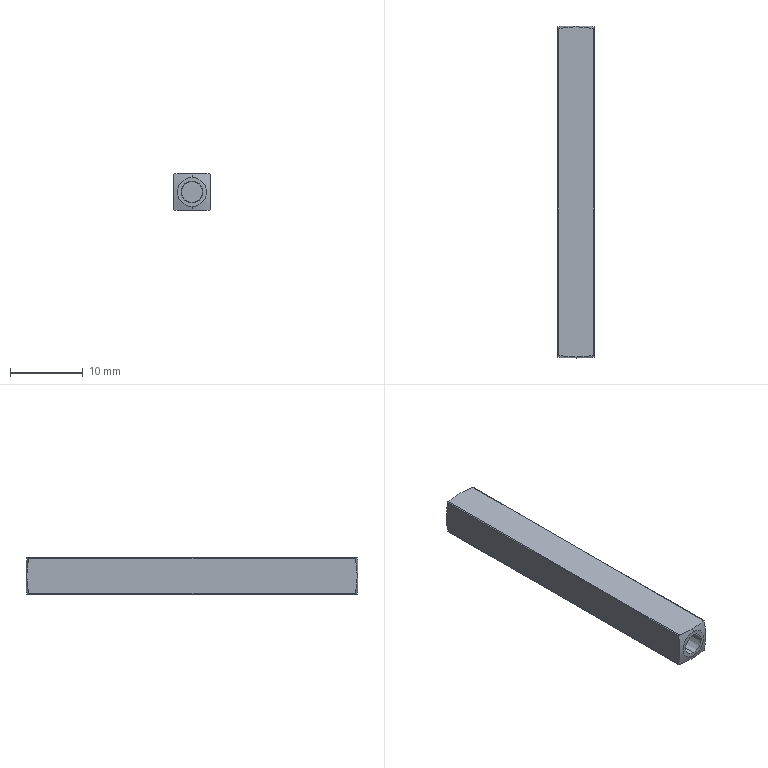Part | STEP file | PCS-C17C-1-2_1_2.stp | 1 solid | 22 faces | box 5 x 45.6 x 5 mm | volume 1100 mm3 | plane 12 | cone 6 | cylinder 4 | commonest cylinder face diameters 0.2 x4
STEP:
#1=CARTESIAN_POINT('',(0.,5.3,1.454));
#2=VERTEX_POINT('',#1);
#3=CARTESIAN_POINT('',(0.,0.,1.5));
#4=VERTEX_POINT('',#3);
#5=CARTESIAN_POINT('',(0.,5.3,1.454));
#6=DIRECTION('',(0.,-1.,0.008727));
#7=VECTOR('',#6,1000.);
#8=LINE('',#5,#7);
#9=EDGE_CURVE('',#2,#4,#8,.T.);
#10=ORIENTED_EDGE('',*,*,#9,.T.);
#11=CARTESIAN_POINT('',(0.,0.,-1.5));
#12=VERTEX_POINT('',#11);
#13=CARTESIAN_POINT('',(0.,0.,0.));
#14=DIRECTION('',(0.,-1.,0.));
#15=DIRECTION('',(0.,0.,1.));
#16=AXIS2_PLACEMENT_3D('',#13,#14,#15);
#17=CIRCLE('',#16,1.5);
#18=EDGE_CURVE('',#4,#12,#17,.T.);
#19=ORIENTED_EDGE('',*,*,#18,.T.);
#20=CARTESIAN_POINT('',(0.,5.3,-1.454));
#21=VERTEX_POINT('',#20);
#22=CARTESIAN_POINT('',(0.,0.,-1.5));
#23=DIRECTION('',(0.,1.,0.008727));
#24=VECTOR('',#23,1000.);
#25=LINE('',#22,#24);
#26=EDGE_CURVE('',#12,#21,#25,.T.);
#27=ORIENTED_EDGE('',*,*,#26,.T.);
#28=CARTESIAN_POINT('',(0.,5.3,0.));
#29=DIRECTION('',(0.,1.,0.));
#30=DIRECTION('',(0.,0.,-1.));
#31=AXIS2_PLACEMENT_3D('',#28,#29,#30);
#32=CIRCLE('',#31,1.454);
#33=EDGE_CURVE('',#21,#2,#32,.T.);
#34=ORIENTED_EDGE('',*,*,#33,.T.);
#35=EDGE_LOOP('',(#10,#19,#27,#34));
#36=FACE_OUTER_BOUND('',#35,.T.);
#37=CARTESIAN_POINT('',(0.,2.65,0.));
#38=DIRECTION('',(0.,-1.,0.));
#39=DIRECTION('',(0.,0.,-1.));
#40=AXIS2_PLACEMENT_3D('',#37,#38,#39);
#41=CONICAL_SURFACE('',#40,1.477,0.008727);
#42=ADVANCED_FACE('',(#36),#41,.F.);
#43=ORIENTED_EDGE('',*,*,#33,.F.);
#44=CARTESIAN_POINT('',(0.,5.3,0.));
#45=DIRECTION('',(0.,1.,0.));
#46=DIRECTION('',(0.,0.,1.));
#47=AXIS2_PLACEMENT_3D('',#44,#45,#46);
#48=CIRCLE('',#47,1.454);
#49=EDGE_CURVE('',#2,#21,#48,.T.);
#50=ORIENTED_EDGE('',*,*,#49,.F.);
#51=EDGE_LOOP('',(#43,#50));
#52=FACE_OUTER_BOUND('',#51,.T.);
#53=CARTESIAN_POINT('',(0.,5.3,0.));
#54=DIRECTION('',(0.,-1.,0.));
#55=DIRECTION('',(0.,0.,-1.));
#56=AXIS2_PLACEMENT_3D('',#53,#54,#55);
#57=PLANE('',#56);
#58=ADVANCED_FACE('',(#52),#57,.T.);
#59=ORIENTED_EDGE('',*,*,#49,.T.);
#60=ORIENTED_EDGE('',*,*,#26,.F.);
#61=CARTESIAN_POINT('',(0.,0.,0.));
#62=DIRECTION('',(0.,-1.,0.));
#63=DIRECTION('',(0.,0.,-1.));
#64=AXIS2_PLACEMENT_3D('',#61,#62,#63);
#65=CIRCLE('',#64,1.5);
#66=EDGE_CURVE('',#12,#4,#65,.T.);
#67=ORIENTED_EDGE('',*,*,#66,.T.);
#68=ORIENTED_EDGE('',*,*,#9,.F.);
#69=EDGE_LOOP('',(#59,#60,#67,#68));
#70=FACE_OUTER_BOUND('',#69,.T.);
#71=CARTESIAN_POINT('',(0.,2.65,0.));
#72=DIRECTION('',(0.,-1.,0.));
#73=DIRECTION('',(0.,0.,-1.));
#74=AXIS2_PLACEMENT_3D('',#71,#72,#73);
#75=CONICAL_SURFACE('',#74,1.477,0.008727);
#76=ADVANCED_FACE('',(#70),#75,.F.);
#77=CARTESIAN_POINT('',(0.,0.,2.));
#78=VERTEX_POINT('',#77);
#79=CARTESIAN_POINT('',(0.,0.,-2.));
#80=VERTEX_POINT('',#79);
#81=CARTESIAN_POINT('',(0.,0.,0.));
#82=DIRECTION('',(0.,1.,0.));
#83=DIRECTION('',(0.,0.,1.));
#84=AXIS2_PLACEMENT_3D('',#81,#82,#83);
#85=CIRCLE('',#84,2.);
#86=EDGE_CURVE('',#78,#80,#85,.T.);
#87=ORIENTED_EDGE('',*,*,#86,.F.);
#88=CARTESIAN_POINT('',(0.,0.,0.));
#89=DIRECTION('',(0.,1.,0.));
#90=DIRECTION('',(0.,0.,-1.));
#91=AXIS2_PLACEMENT_3D('',#88,#89,#90);
#92=CIRCLE('',#91,2.);
#93=EDGE_CURVE('',#80,#78,#92,.T.);
#94=ORIENTED_EDGE('',*,*,#93,.F.);
#95=EDGE_LOOP('',(#87,#94));
#96=FACE_OUTER_BOUND('',#95,.T.);
#97=ORIENTED_EDGE('',*,*,#18,.F.);
#98=ORIENTED_EDGE('',*,*,#66,.F.);
#99=EDGE_LOOP('',(#97,#98));
#100=FACE_BOUND('',#99,.T.);
#101=CARTESIAN_POINT('',(-2.4,0.,-2.4));
#102=DIRECTION('',(0.,-1.,0.));
#103=DIRECTION('',(0.,0.,-1.));
#104=AXIS2_PLACEMENT_3D('',#101,#102,#103);
#105=PLANE('',#104);
#106=ADVANCED_FACE('',(#96,#100),#105,.T.);
#107=ORIENTED_EDGE('',*,*,#93,.T.);
#108=CARTESIAN_POINT('',(0.,0.125,2.5));
#109=VERTEX_POINT('',#108);
#110=CARTESIAN_POINT('',(0.,0.125,2.5));
#111=DIRECTION('',(0.,-0.2425,-0.9701));
#112=VECTOR('',#111,1000.);
#113=LINE('',#110,#112);
#114=EDGE_CURVE('',#109,#78,#113,.T.);
#115=ORIENTED_EDGE('',*,*,#114,.F.);
#116=CARTESIAN_POINT('',(-2.4,0.3664,2.5));
#117=VERTEX_POINT('',#116);
#118=CARTESIAN_POINT('',(-2.4,0.3664,2.5));
#119=CARTESIAN_POINT('',(-2.171,0.3267,2.5));
#120=CARTESIAN_POINT('',(-1.844,0.2747,2.5));
#121=CARTESIAN_POINT('',(-1.493,0.2276,2.5));
#122=CARTESIAN_POINT('',(-1.326,0.2073,2.5));
#123=CARTESIAN_POINT('',(-1.244,0.198,2.5));
#124=CARTESIAN_POINT('',(-1.209,0.1942,2.5));
#125=CARTESIAN_POINT('',(-1.186,0.1918,2.5));
#126=CARTESIAN_POINT('',(-1.176,0.1907,2.5));
#127=CARTESIAN_POINT('',(-0.7566,0.1464,2.5));
#128=CARTESIAN_POINT('',(-0.3689,0.125,2.5));
#129=CARTESIAN_POINT('',(0.,0.125,2.5));
#130=B_SPLINE_CURVE_WITH_KNOTS('',3,(#118,#119,#120,#121,#122,#123,#124,#125,#126,#127,#128,#129),.UNSPECIFIED.,.F.,.F.,(4,1,1,1,1,2,2,4),(0.,0.25,0.375,0.4375,0.4688,0.4844,0.5,1.),.UNSPECIFIED.);
#131=EDGE_CURVE('',#117,#109,#130,.T.);
#132=ORIENTED_EDGE('',*,*,#131,.F.);
#133=CARTESIAN_POINT('',(-2.5,0.3664,2.4));
#134=VERTEX_POINT('',#133);
#135=CARTESIAN_POINT('',(-2.5,0.3664,2.4));
#136=CARTESIAN_POINT('',(-2.5,0.3709,2.426));
#137=CARTESIAN_POINT('',(-2.489,0.3732,2.452));
#138=CARTESIAN_POINT('',(-2.452,0.3732,2.489));
#139=CARTESIAN_POINT('',(-2.426,0.3709,2.5));
#140=CARTESIAN_POINT('',(-2.4,0.3664,2.5));
#141=B_SPLINE_CURVE_WITH_KNOTS('',3,(#135,#136,#137,#138,#139,#140),.UNSPECIFIED.,.F.,.F.,(4,2,4),(0.,0.5,1.),.UNSPECIFIED.);
#142=EDGE_CURVE('',#134,#117,#141,.T.);
#143=ORIENTED_EDGE('',*,*,#142,.F.);
#144=CARTESIAN_POINT('',(-2.5,0.3664,-2.4));
#145=VERTEX_POINT('',#144);
#146=CARTESIAN_POINT('',(-2.5,0.3664,-2.4));
#147=CARTESIAN_POINT('',(-2.5,0.327,-2.173));
#148=CARTESIAN_POINT('',(-2.5,0.2755,-1.849));
#149=CARTESIAN_POINT('',(-2.5,0.2285,-1.5));
#150=CARTESIAN_POINT('',(-2.5,0.2083,-1.334));
#151=CARTESIAN_POINT('',(-2.5,0.199,-1.252));
#152=CARTESIAN_POINT('',(-2.5,0.1952,-1.218));
#153=CARTESIAN_POINT('',(-2.5,0.1927,-1.195));
#154=CARTESIAN_POINT('',(-2.5,0.1916,-1.185));
#155=CARTESIAN_POINT('',(-2.5,0.1688,-0.9703));
#156=CARTESIAN_POINT('',(-2.5,0.1526,-0.7728));
#157=CARTESIAN_POINT('',(-2.5,0.1309,-0.3869));
#158=CARTESIAN_POINT('',(-2.5,0.1253,-0.2006));
#159=CARTESIAN_POINT('',(-2.5,0.1247,0.1713));
#160=CARTESIAN_POINT('',(-2.5,0.1325,0.4571));
#161=CARTESIAN_POINT('',(-2.5,0.1558,0.8028));
#162=CARTESIAN_POINT('',(-2.5,0.171,0.9786));
#163=CARTESIAN_POINT('',(-2.5,0.1795,1.067));
#164=CARTESIAN_POINT('',(-2.5,0.1834,1.106));
#165=CARTESIAN_POINT('',(-2.5,0.186,1.131));
#166=CARTESIAN_POINT('',(-2.5,0.1874,1.145));
#167=CARTESIAN_POINT('',(-2.5,0.2272,1.524));
#168=CARTESIAN_POINT('',(-2.5,0.2865,1.939));
#169=CARTESIAN_POINT('',(-2.5,0.3664,2.4));
#170=B_SPLINE_CURVE_WITH_KNOTS('',3,(#146,#147,#148,#149,#150,#151,#152,#153,#154,#155,#156,#157,#158,#159,#160,#161,#162,#163,#164,#165,#166,#167,#168,#169),.UNSPECIFIED.,.F.,.F.,(4,1,1,1,1,2,2,2,2,1,1,1,1,2,2,4),(0.,0.125,0.1875,0.2187,0.2344,0.2422,0.25,0.375,0.5,0.625,0.6875,0.7187,0.7344,0.7422,0.75,1.),.UNSPECIFIED.);
#171=EDGE_CURVE('',#145,#134,#170,.T.);
#172=ORIENTED_EDGE('',*,*,#171,.F.);
#173=CARTESIAN_POINT('',(-2.4,0.3664,-2.5));
#174=VERTEX_POINT('',#173);
#175=CARTESIAN_POINT('',(-2.4,0.3664,-2.5));
#176=CARTESIAN_POINT('',(-2.426,0.3709,-2.5));
#177=CARTESIAN_POINT('',(-2.452,0.3732,-2.489));
#178=CARTESIAN_POINT('',(-2.489,0.3732,-2.452));
#179=CARTESIAN_POINT('',(-2.5,0.3709,-2.426));
#180=CARTESIAN_POINT('',(-2.5,0.3664,-2.4));
#181=B_SPLINE_CURVE_WITH_KNOTS('',3,(#175,#176,#177,#178,#179,#180),.UNSPECIFIED.,.F.,.F.,(4,2,4),(0.,0.5,1.),.UNSPECIFIED.);
#182=EDGE_CURVE('',#174,#145,#181,.T.);
#183=ORIENTED_EDGE('',*,*,#182,.F.);
#184=CARTESIAN_POINT('',(0.,0.125,-2.5));
#185=VERTEX_POINT('',#184);
#186=CARTESIAN_POINT('',(0.,0.125,-2.5));
#187=CARTESIAN_POINT('',(-0.1844,0.125,-2.5));
#188=CARTESIAN_POINT('',(-0.4682,0.1331,-2.5));
#189=CARTESIAN_POINT('',(-0.8119,0.1565,-2.5));
#190=CARTESIAN_POINT('',(-0.9868,0.1718,-2.5));
#191=CARTESIAN_POINT('',(-1.075,0.1803,-2.5));
#192=CARTESIAN_POINT('',(-1.113,0.1841,-2.5));
#193=CARTESIAN_POINT('',(-1.138,0.1867,-2.5));
#194=CARTESIAN_POINT('',(-1.152,0.1882,-2.5));
#195=CARTESIAN_POINT('',(-1.529,0.2279,-2.5));
#196=CARTESIAN_POINT('',(-1.941,0.2869,-2.5));
#197=CARTESIAN_POINT('',(-2.4,0.3664,-2.5));
#198=B_SPLINE_CURVE_WITH_KNOTS('',3,(#186,#187,#188,#189,#190,#191,#192,#193,#194,#195,#196,#197),.UNSPECIFIED.,.F.,.F.,(4,1,1,1,1,2,2,4),(0.,0.25,0.375,0.4375,0.4687,0.4844,0.5,1.),.UNSPECIFIED.);
#199=EDGE_CURVE('',#185,#174,#198,.T.);
#200=ORIENTED_EDGE('',*,*,#199,.F.);
#201=CARTESIAN_POINT('',(0.,0.,-2.));
#202=DIRECTION('',(0.,0.2425,-0.9701));
#203=VECTOR('',#202,1000.);
#204=LINE('',#201,#203);
#205=EDGE_CURVE('',#80,#185,#204,.T.);
#206=ORIENTED_EDGE('',*,*,#205,.F.);
#207=EDGE_LOOP('',(#107,#115,#132,#143,#172,#183,#200,#206));
#208=FACE_OUTER_BOUND('',#207,.T.);
#209=CARTESIAN_POINT('',(0.,0.1868,0.));
#210=DIRECTION('',(0.,1.,0.));
#211=DIRECTION('',(0.,0.,1.));
#212=AXIS2_PLACEMENT_3D('',#209,#210,#211);
#213=CONICAL_SURFACE('',#212,2.747,1.326);
#214=ADVANCED_FACE('',(#208),#213,.T.);
#215=ORIENTED_EDGE('',*,*,#205,.T.);
#216=CARTESIAN_POINT('',(2.4,0.3664,-2.5));
#217=VERTEX_POINT('',#216);
#218=CARTESIAN_POINT('',(2.4,0.3664,-2.5));
#219=CARTESIAN_POINT('',(2.171,0.3267,-2.5));
#220=CARTESIAN_POINT('',(1.844,0.2747,-2.5));
#221=CARTESIAN_POINT('',(1.493,0.2276,-2.5));
#222=CARTESIAN_POINT('',(1.326,0.2073,-2.5));
#223=CARTESIAN_POINT('',(1.244,0.198,-2.5));
#224=CARTESIAN_POINT('',(1.209,0.1942,-2.5));
#225=CARTESIAN_POINT('',(1.186,0.1918,-2.5));
#226=CARTESIAN_POINT('',(1.176,0.1907,-2.5));
#227=CARTESIAN_POINT('',(0.7566,0.1464,-2.5));
#228=CARTESIAN_POINT('',(0.3689,0.125,-2.5));
#229=CARTESIAN_POINT('',(0.,0.125,-2.5));
#230=B_SPLINE_CURVE_WITH_KNOTS('',3,(#218,#219,#220,#221,#222,#223,#224,#225,#226,#227,#228,#229),.UNSPECIFIED.,.F.,.F.,(4,1,1,1,1,2,2,4),(0.,0.25,0.375,0.4375,0.4688,0.4844,0.5,1.),.UNSPECIFIED.);
#231=EDGE_CURVE('',#217,#185,#230,.T.);
#232=ORIENTED_EDGE('',*,*,#231,.F.);
#233=CARTESIAN_POINT('',(2.5,0.3664,-2.4));
#234=VERTEX_POINT('',#233);
#235=CARTESIAN_POINT('',(2.4,0.3664,-2.5));
#236=CARTESIAN_POINT('',(2.413,0.3687,-2.5));
#237=CARTESIAN_POINT('',(2.44,0.3723,-2.495));
#238=CARTESIAN_POINT('',(2.473,0.3742,-2.472));
#239=CARTESIAN_POINT('',(2.495,0.3722,-2.439));
#240=CARTESIAN_POINT('',(2.5,0.3686,-2.413));
#241=CARTESIAN_POINT('',(2.5,0.3664,-2.4));
#242=B_SPLINE_CURVE_WITH_KNOTS('',3,(#235,#236,#237,#238,#239,#240,#241),.UNSPECIFIED.,.F.,.F.,(4,1,1,1,4),(0.,0.25,0.5,0.75,1.),.UNSPECIFIED.);
#243=EDGE_CURVE('',#217,#234,#242,.T.);
#244=ORIENTED_EDGE('',*,*,#243,.T.);
#245=CARTESIAN_POINT('',(2.5,0.3664,2.4));
#246=VERTEX_POINT('',#245);
#247=CARTESIAN_POINT('',(2.5,0.3664,2.4));
#248=CARTESIAN_POINT('',(2.5,0.327,2.173));
#249=CARTESIAN_POINT('',(2.5,0.2755,1.849));
#250=CARTESIAN_POINT('',(2.5,0.2286,1.501));
#251=CARTESIAN_POINT('',(2.5,0.2084,1.334));
#252=CARTESIAN_POINT('',(2.5,0.1991,1.253));
#253=CARTESIAN_POINT('',(2.5,0.1953,1.219));
#254=CARTESIAN_POINT('',(2.5,0.1928,1.196));
#255=CARTESIAN_POINT('',(2.5,0.1917,1.186));
#256=CARTESIAN_POINT('',(2.5,0.1689,0.9709));
#257=CARTESIAN_POINT('',(2.5,0.1527,0.7734));
#258=CARTESIAN_POINT('',(2.5,0.1309,0.3874));
#259=CARTESIAN_POINT('',(2.5,0.1253,0.201));
#260=CARTESIAN_POINT('',(2.5,0.1247,-0.1709));
#261=CARTESIAN_POINT('',(2.5,0.1325,-0.4568));
#262=CARTESIAN_POINT('',(2.5,0.1558,-0.8026));
#263=CARTESIAN_POINT('',(2.5,0.171,-0.9785));
#264=CARTESIAN_POINT('',(2.5,0.1795,-1.067));
#265=CARTESIAN_POINT('',(2.5,0.1834,-1.105));
#266=CARTESIAN_POINT('',(2.5,0.186,-1.131));
#267=CARTESIAN_POINT('',(2.5,0.1874,-1.145));
#268=CARTESIAN_POINT('',(2.5,0.2272,-1.524));
#269=CARTESIAN_POINT('',(2.5,0.2865,-1.938));
#270=CARTESIAN_POINT('',(2.5,0.3664,-2.4));
#271=B_SPLINE_CURVE_WITH_KNOTS('',3,(#247,#248,#249,#250,#251,#252,#253,#254,#255,#256,#257,#258,#259,#260,#261,#262,#263,#264,#265,#266,#267,#268,#269,#270),.UNSPECIFIED.,.F.,.F.,(4,1,1,1,1,2,2,2,2,1,1,1,1,2,2,4),(0.,0.125,0.1875,0.2188,0.2344,0.2422,0.25,0.375,0.5,0.625,0.6875,0.7188,0.7344,0.7422,0.75,1.),.UNSPECIFIED.);
#272=EDGE_CURVE('',#246,#234,#271,.T.);
#273=ORIENTED_EDGE('',*,*,#272,.F.);
#274=CARTESIAN_POINT('',(2.4,0.3664,2.5));
#275=VERTEX_POINT('',#274);
#276=CARTESIAN_POINT('',(2.5,0.3664,2.4));
#277=CARTESIAN_POINT('',(2.5,0.3687,2.413));
#278=CARTESIAN_POINT('',(2.495,0.3723,2.44));
#279=CARTESIAN_POINT('',(2.472,0.3742,2.473));
#280=CARTESIAN_POINT('',(2.439,0.3722,2.495));
#281=CARTESIAN_POINT('',(2.413,0.3686,2.5));
#282=CARTESIAN_POINT('',(2.4,0.3664,2.5));
#283=B_SPLINE_CURVE_WITH_KNOTS('',3,(#276,#277,#278,#279,#280,#281,#282),.UNSPECIFIED.,.F.,.F.,(4,1,1,1,4),(0.,0.25,0.5,0.75,1.),.UNSPECIFIED.);
#284=EDGE_CURVE('',#246,#275,#283,.T.);
#285=ORIENTED_EDGE('',*,*,#284,.T.);
#286=CARTESIAN_POINT('',(0.,0.125,2.5));
#287=CARTESIAN_POINT('',(0.1844,0.125,2.5));
#288=CARTESIAN_POINT('',(0.4682,0.1331,2.5));
#289=CARTESIAN_POINT('',(0.8118,0.1565,2.5));
#290=CARTESIAN_POINT('',(0.9868,0.1718,2.5));
#291=CARTESIAN_POINT('',(1.075,0.1803,2.5));
#292=CARTESIAN_POINT('',(1.113,0.1841,2.5));
#293=CARTESIAN_POINT('',(1.138,0.1867,2.5));
#294=CARTESIAN_POINT('',(1.152,0.1882,2.5));
#295=CARTESIAN_POINT('',(1.529,0.2279,2.5));
#296=CARTESIAN_POINT('',(1.941,0.2869,2.5));
#297=CARTESIAN_POINT('',(2.4,0.3664,2.5));
#298=B_SPLINE_CURVE_WITH_KNOTS('',3,(#286,#287,#288,#289,#290,#291,#292,#293,#294,#295,#296,#297),.UNSPECIFIED.,.F.,.F.,(4,1,1,1,1,2,2,4),(0.,0.25,0.375,0.4375,0.4688,0.4844,0.5,1.),.UNSPECIFIED.);
#299=EDGE_CURVE('',#109,#275,#298,.T.);
#300=ORIENTED_EDGE('',*,*,#299,.F.);
#301=ORIENTED_EDGE('',*,*,#114,.T.);
#302=ORIENTED_EDGE('',*,*,#86,.T.);
#303=EDGE_LOOP('',(#215,#232,#244,#273,#285,#300,#301,#302));
#304=FACE_OUTER_BOUND('',#303,.T.);
#305=CARTESIAN_POINT('',(0.,0.1868,0.));
#306=DIRECTION('',(0.,1.,0.));
#307=DIRECTION('',(0.,0.,1.));
#308=AXIS2_PLACEMENT_3D('',#305,#306,#307);
#309=CONICAL_SURFACE('',#308,2.747,1.326);
#310=ADVANCED_FACE('',(#304),#309,.T.);
#311=ORIENTED_EDGE('',*,*,#131,.T.);
#312=ORIENTED_EDGE('',*,*,#299,.T.);
#313=CARTESIAN_POINT('',(2.4,45.234,2.5));
#314=VERTEX_POINT('',#313);
#315=CARTESIAN_POINT('',(2.4,45.234,2.5));
#316=DIRECTION('',(0.,-1.,0.));
#317=VECTOR('',#316,1000.);
#318=LINE('',#315,#317);
#319=EDGE_CURVE('',#314,#275,#318,.T.);
#320=ORIENTED_EDGE('',*,*,#319,.F.);
#321=CARTESIAN_POINT('',(0.,45.475,2.5));
#322=VERTEX_POINT('',#321);
#323=CARTESIAN_POINT('',(2.4,45.234,2.5));
#324=CARTESIAN_POINT('',(2.171,45.273,2.5));
#325=CARTESIAN_POINT('',(1.844,45.325,2.5));
#326=CARTESIAN_POINT('',(1.493,45.372,2.5));
#327=CARTESIAN_POINT('',(1.326,45.393,2.5));
#328=CARTESIAN_POINT('',(1.244,45.402,2.5));
#329=CARTESIAN_POINT('',(1.209,45.406,2.5));
#330=CARTESIAN_POINT('',(1.186,45.408,2.5));
#331=CARTESIAN_POINT('',(1.176,45.409,2.5));
#332=CARTESIAN_POINT('',(0.7566,45.454,2.5));
#333=CARTESIAN_POINT('',(0.3689,45.475,2.5));
#334=CARTESIAN_POINT('',(0.,45.475,2.5));
#335=B_SPLINE_CURVE_WITH_KNOTS('',3,(#323,#324,#325,#326,#327,#328,#329,#330,#331,#332,#333,#334),.UNSPECIFIED.,.F.,.F.,(4,1,1,1,1,2,2,4),(0.,0.25,0.375,0.4375,0.4688,0.4844,0.5,1.),.UNSPECIFIED.);
#336=EDGE_CURVE('',#314,#322,#335,.T.);
#337=ORIENTED_EDGE('',*,*,#336,.T.);
#338=CARTESIAN_POINT('',(-2.4,45.234,2.5));
#339=VERTEX_POINT('',#338);
#340=CARTESIAN_POINT('',(0.,45.475,2.5));
#341=CARTESIAN_POINT('',(-0.1844,45.475,2.5));
#342=CARTESIAN_POINT('',(-0.4682,45.467,2.5));
#343=CARTESIAN_POINT('',(-0.8119,45.443,2.5));
#344=CARTESIAN_POINT('',(-0.9868,45.428,2.5));
#345=CARTESIAN_POINT('',(-1.075,45.42,2.5));
#346=CARTESIAN_POINT('',(-1.113,45.416,2.5));
#347=CARTESIAN_POINT('',(-1.138,45.413,2.5));
#348=CARTESIAN_POINT('',(-1.152,45.412,2.5));
#349=CARTESIAN_POINT('',(-1.529,45.372,2.5));
#350=CARTESIAN_POINT('',(-1.941,45.313,2.5));
#351=CARTESIAN_POINT('',(-2.4,45.234,2.5));
#352=B_SPLINE_CURVE_WITH_KNOTS('',3,(#340,#341,#342,#343,#344,#345,#346,#347,#348,#349,#350,#351),.UNSPECIFIED.,.F.,.F.,(4,1,1,1,1,2,2,4),(0.,0.25,0.375,0.4375,0.4687,0.4844,0.5,1.),.UNSPECIFIED.);
#353=EDGE_CURVE('',#322,#339,#352,.T.);
#354=ORIENTED_EDGE('',*,*,#353,.T.);
#355=CARTESIAN_POINT('',(-2.4,0.3664,2.5));
#356=DIRECTION('',(0.,1.,0.));
#357=VECTOR('',#356,1000.);
#358=LINE('',#355,#357);
#359=EDGE_CURVE('',#117,#339,#358,.T.);
#360=ORIENTED_EDGE('',*,*,#359,.F.);
#361=EDGE_LOOP('',(#311,#312,#320,#337,#354,#360));
#362=FACE_OUTER_BOUND('',#361,.T.);
#363=CARTESIAN_POINT('',(-2.4,45.6,2.5));
#364=DIRECTION('',(0.,0.,-1.));
#365=DIRECTION('',(0.,-1.,0.));
#366=AXIS2_PLACEMENT_3D('',#363,#364,#365);
#367=PLANE('',#366);
#368=ADVANCED_FACE('',(#362),#367,.F.);
#369=ORIENTED_EDGE('',*,*,#142,.T.);
#370=ORIENTED_EDGE('',*,*,#359,.T.);
#371=CARTESIAN_POINT('',(-2.5,45.234,2.4));
#372=VERTEX_POINT('',#371);
#373=CARTESIAN_POINT('',(-2.4,45.234,2.5));
#374=CARTESIAN_POINT('',(-2.426,45.229,2.5));
#375=CARTESIAN_POINT('',(-2.452,45.227,2.489));
#376=CARTESIAN_POINT('',(-2.489,45.227,2.452));
#377=CARTESIAN_POINT('',(-2.5,45.229,2.426));
#378=CARTESIAN_POINT('',(-2.5,45.234,2.4));
#379=B_SPLINE_CURVE_WITH_KNOTS('',3,(#373,#374,#375,#376,#377,#378),.UNSPECIFIED.,.F.,.F.,(4,2,4),(0.,0.5,1.),.UNSPECIFIED.);
#380=EDGE_CURVE('',#339,#372,#379,.T.);
#381=ORIENTED_EDGE('',*,*,#380,.T.);
#382=CARTESIAN_POINT('',(-2.5,45.234,2.4));
#383=DIRECTION('',(0.,-1.,0.));
#384=VECTOR('',#383,1000.);
#385=LINE('',#382,#384);
#386=EDGE_CURVE('',#372,#134,#385,.T.);
#387=ORIENTED_EDGE('',*,*,#386,.T.);
#388=EDGE_LOOP('',(#369,#370,#381,#387));
#389=FACE_OUTER_BOUND('',#388,.T.);
#390=CARTESIAN_POINT('',(-2.4,0.09718,2.4));
#391=DIRECTION('',(0.,-1.,0.));
#392=DIRECTION('',(0.,0.,-1.));
#393=AXIS2_PLACEMENT_3D('',#390,#391,#392);
#394=CYLINDRICAL_SURFACE('',#393,0.1);
#395=ADVANCED_FACE('',(#389),#394,.T.);
#396=ORIENTED_EDGE('',*,*,#171,.T.);
#397=ORIENTED_EDGE('',*,*,#386,.F.);
#398=CARTESIAN_POINT('',(-2.5,45.234,-2.4));
#399=VERTEX_POINT('',#398);
#400=CARTESIAN_POINT('',(-2.5,45.234,2.4));
#401=CARTESIAN_POINT('',(-2.5,45.273,2.173));
#402=CARTESIAN_POINT('',(-2.5,45.324,1.849));
#403=CARTESIAN_POINT('',(-2.5,45.371,1.501));
#404=CARTESIAN_POINT('',(-2.5,45.392,1.334));
#405=CARTESIAN_POINT('',(-2.5,45.401,1.253));
#406=CARTESIAN_POINT('',(-2.5,45.405,1.219));
#407=CARTESIAN_POINT('',(-2.5,45.407,1.196));
#408=CARTESIAN_POINT('',(-2.5,45.408,1.186));
#409=CARTESIAN_POINT('',(-2.5,45.431,0.9709));
#410=CARTESIAN_POINT('',(-2.5,45.447,0.7734));
#411=CARTESIAN_POINT('',(-2.5,45.469,0.3874));
#412=CARTESIAN_POINT('',(-2.5,45.475,0.201));
#413=CARTESIAN_POINT('',(-2.5,45.475,-0.1709));
#414=CARTESIAN_POINT('',(-2.5,45.468,-0.4568));
#415=CARTESIAN_POINT('',(-2.5,45.444,-0.8026));
#416=CARTESIAN_POINT('',(-2.5,45.429,-0.9785));
#417=CARTESIAN_POINT('',(-2.5,45.42,-1.067));
#418=CARTESIAN_POINT('',(-2.5,45.417,-1.105));
#419=CARTESIAN_POINT('',(-2.5,45.414,-1.131));
#420=CARTESIAN_POINT('',(-2.5,45.413,-1.145));
#421=CARTESIAN_POINT('',(-2.5,45.373,-1.524));
#422=CARTESIAN_POINT('',(-2.5,45.314,-1.938));
#423=CARTESIAN_POINT('',(-2.5,45.234,-2.4));
#424=B_SPLINE_CURVE_WITH_KNOTS('',3,(#400,#401,#402,#403,#404,#405,#406,#407,#408,#409,#410,#411,#412,#413,#414,#415,#416,#417,#418,#419,#420,#421,#422,#423),.UNSPECIFIED.,.F.,.F.,(4,1,1,1,1,2,2,2,2,1,1,1,1,2,2,4),(0.,0.125,0.1875,0.2188,0.2344,0.2422,0.25,0.375,0.5,0.625,0.6875,0.7188,0.7344,0.7422,0.75,1.),.UNSPECIFIED.);
#425=EDGE_CURVE('',#372,#399,#424,.T.);
#426=ORIENTED_EDGE('',*,*,#425,.T.);
#427=CARTESIAN_POINT('',(-2.5,0.3664,-2.4));
#428=DIRECTION('',(0.,1.,0.));
#429=VECTOR('',#428,1000.);
#430=LINE('',#427,#429);
#431=EDGE_CURVE('',#145,#399,#430,.T.);
#432=ORIENTED_EDGE('',*,*,#431,.F.);
#433=EDGE_LOOP('',(#396,#397,#426,#432));
#434=FACE_OUTER_BOUND('',#433,.T.);
#435=CARTESIAN_POINT('',(-2.5,45.6,-2.4));
#436=DIRECTION('',(1.,0.,0.));
#437=DIRECTION('',(0.,1.,0.));
#438=AXIS2_PLACEMENT_3D('',#435,#436,#437);
#439=PLANE('',#438);
#440=ADVANCED_FACE('',(#434),#439,.F.);
#441=ORIENTED_EDGE('',*,*,#182,.T.);
#442=ORIENTED_EDGE('',*,*,#431,.T.);
#443=CARTESIAN_POINT('',(-2.4,45.234,-2.5));
#444=VERTEX_POINT('',#443);
#445=CARTESIAN_POINT('',(-2.5,45.234,-2.4));
#446=CARTESIAN_POINT('',(-2.5,45.229,-2.426));
#447=CARTESIAN_POINT('',(-2.489,45.227,-2.452));
#448=CARTESIAN_POINT('',(-2.452,45.227,-2.489));
#449=CARTESIAN_POINT('',(-2.426,45.229,-2.5));
#450=CARTESIAN_POINT('',(-2.4,45.234,-2.5));
#451=B_SPLINE_CURVE_WITH_KNOTS('',3,(#445,#446,#447,#448,#449,#450),.UNSPECIFIED.,.F.,.F.,(4,2,4),(0.,0.5,1.),.UNSPECIFIED.);
#452=EDGE_CURVE('',#399,#444,#451,.T.);
#453=ORIENTED_EDGE('',*,*,#452,.T.);
#454=CARTESIAN_POINT('',(-2.4,45.234,-2.5));
#455=DIRECTION('',(0.,-1.,0.));
#456=VECTOR('',#455,1000.);
#457=LINE('',#454,#456);
#458=EDGE_CURVE('',#444,#174,#457,.T.);
#459=ORIENTED_EDGE('',*,*,#458,.T.);
#460=EDGE_LOOP('',(#441,#442,#453,#459));
#461=FACE_OUTER_BOUND('',#460,.T.);
#462=CARTESIAN_POINT('',(-2.4,0.09718,-2.4));
#463=DIRECTION('',(0.,-1.,0.));
#464=DIRECTION('',(0.,0.,-1.));
#465=AXIS2_PLACEMENT_3D('',#462,#463,#464);
#466=CYLINDRICAL_SURFACE('',#465,0.1);
#467=ADVANCED_FACE('',(#461),#466,.T.);
#468=ORIENTED_EDGE('',*,*,#231,.T.);
#469=ORIENTED_EDGE('',*,*,#199,.T.);
#470=ORIENTED_EDGE('',*,*,#458,.F.);
#471=CARTESIAN_POINT('',(0.,45.475,-2.5));
#472=VERTEX_POINT('',#471);
#473=CARTESIAN_POINT('',(-2.4,45.234,-2.5));
#474=CARTESIAN_POINT('',(-2.171,45.273,-2.5));
#475=CARTESIAN_POINT('',(-1.844,45.325,-2.5));
#476=CARTESIAN_POINT('',(-1.493,45.372,-2.5));
#477=CARTESIAN_POINT('',(-1.326,45.393,-2.5));
#478=CARTESIAN_POINT('',(-1.244,45.402,-2.5));
#479=CARTESIAN_POINT('',(-1.209,45.406,-2.5));
#480=CARTESIAN_POINT('',(-1.186,45.408,-2.5));
#481=CARTESIAN_POINT('',(-1.176,45.409,-2.5));
#482=CARTESIAN_POINT('',(-0.7566,45.454,-2.5));
#483=CARTESIAN_POINT('',(-0.3689,45.475,-2.5));
#484=CARTESIAN_POINT('',(0.,45.475,-2.5));
#485=B_SPLINE_CURVE_WITH_KNOTS('',3,(#473,#474,#475,#476,#477,#478,#479,#480,#481,#482,#483,#484),.UNSPECIFIED.,.F.,.F.,(4,1,1,1,1,2,2,4),(0.,0.25,0.375,0.4375,0.4687,0.4844,0.5,1.),.UNSPECIFIED.);
#486=EDGE_CURVE('',#444,#472,#485,.T.);
#487=ORIENTED_EDGE('',*,*,#486,.T.);
#488=CARTESIAN_POINT('',(2.4,45.234,-2.5));
#489=VERTEX_POINT('',#488);
#490=CARTESIAN_POINT('',(0.,45.475,-2.5));
#491=CARTESIAN_POINT('',(0.1844,45.475,-2.5));
#492=CARTESIAN_POINT('',(0.4682,45.467,-2.5));
#493=CARTESIAN_POINT('',(0.8118,45.443,-2.5));
#494=CARTESIAN_POINT('',(0.9868,45.428,-2.5));
#495=CARTESIAN_POINT('',(1.075,45.42,-2.5));
#496=CARTESIAN_POINT('',(1.113,45.416,-2.5));
#497=CARTESIAN_POINT('',(1.138,45.413,-2.5));
#498=CARTESIAN_POINT('',(1.152,45.412,-2.5));
#499=CARTESIAN_POINT('',(1.529,45.372,-2.5));
#500=CARTESIAN_POINT('',(1.941,45.313,-2.5));
#501=CARTESIAN_POINT('',(2.4,45.234,-2.5));
#502=B_SPLINE_CURVE_WITH_KNOTS('',3,(#490,#491,#492,#493,#494,#495,#496,#497,#498,#499,#500,#501),.UNSPECIFIED.,.F.,.F.,(4,1,1,1,1,2,2,4),(0.,0.25,0.375,0.4375,0.4687,0.4844,0.5,1.),.UNSPECIFIED.);
#503=EDGE_CURVE('',#472,#489,#502,.T.);
#504=ORIENTED_EDGE('',*,*,#503,.T.);
#505=CARTESIAN_POINT('',(2.4,0.3664,-2.5));
#506=DIRECTION('',(0.,1.,0.));
#507=VECTOR('',#506,1000.);
#508=LINE('',#505,#507);
#509=EDGE_CURVE('',#217,#489,#508,.T.);
#510=ORIENTED_EDGE('',*,*,#509,.F.);
#511=EDGE_LOOP('',(#468,#469,#470,#487,#504,#510));
#512=FACE_OUTER_BOUND('',#511,.T.);
#513=CARTESIAN_POINT('',(-2.4,45.6,-2.5));
#514=DIRECTION('',(0.,0.,1.));
#515=DIRECTION('',(1.,0.,0.));
#516=AXIS2_PLACEMENT_3D('',#513,#514,#515);
#517=PLANE('',#516);
#518=ADVANCED_FACE('',(#512),#517,.F.);
#519=ORIENTED_EDGE('',*,*,#243,.F.);
#520=ORIENTED_EDGE('',*,*,#509,.T.);
#521=CARTESIAN_POINT('',(2.5,45.234,-2.4));
#522=VERTEX_POINT('',#521);
#523=CARTESIAN_POINT('',(2.5,45.234,-2.4));
#524=CARTESIAN_POINT('',(2.5,45.231,-2.413));
#525=CARTESIAN_POINT('',(2.495,45.228,-2.44));
#526=CARTESIAN_POINT('',(2.472,45.226,-2.473));
#527=CARTESIAN_POINT('',(2.439,45.228,-2.495));
#528=CARTESIAN_POINT('',(2.413,45.231,-2.5));
#529=CARTESIAN_POINT('',(2.4,45.234,-2.5));
#530=B_SPLINE_CURVE_WITH_KNOTS('',3,(#523,#524,#525,#526,#527,#528,#529),.UNSPECIFIED.,.F.,.F.,(4,1,1,1,4),(0.,0.25,0.5,0.75,1.),.UNSPECIFIED.);
#531=EDGE_CURVE('',#522,#489,#530,.T.);
#532=ORIENTED_EDGE('',*,*,#531,.F.);
#533=CARTESIAN_POINT('',(2.5,45.234,-2.4));
#534=DIRECTION('',(0.,-1.,0.));
#535=VECTOR('',#534,1000.);
#536=LINE('',#533,#535);
#537=EDGE_CURVE('',#522,#234,#536,.T.);
#538=ORIENTED_EDGE('',*,*,#537,.T.);
#539=EDGE_LOOP('',(#519,#520,#532,#538));
#540=FACE_OUTER_BOUND('',#539,.T.);
#541=CARTESIAN_POINT('',(2.4,0.09718,-2.4));
#542=DIRECTION('',(0.,-1.,0.));
#543=DIRECTION('',(0.,0.,-1.));
#544=AXIS2_PLACEMENT_3D('',#541,#542,#543);
#545=CYLINDRICAL_SURFACE('',#544,0.1);
#546=ADVANCED_FACE('',(#540),#545,.T.);
#547=ORIENTED_EDGE('',*,*,#272,.T.);
#548=ORIENTED_EDGE('',*,*,#537,.F.);
#549=CARTESIAN_POINT('',(2.5,45.234,2.4));
#550=VERTEX_POINT('',#549);
#551=CARTESIAN_POINT('',(2.5,45.234,-2.4));
#552=CARTESIAN_POINT('',(2.5,45.273,-2.173));
#553=CARTESIAN_POINT('',(2.5,45.325,-1.849));
#554=CARTESIAN_POINT('',(2.5,45.371,-1.5));
#555=CARTESIAN_POINT('',(2.5,45.392,-1.334));
#556=CARTESIAN_POINT('',(2.5,45.401,-1.252));
#557=CARTESIAN_POINT('',(2.5,45.405,-1.218));
#558=CARTESIAN_POINT('',(2.5,45.407,-1.195));
#559=CARTESIAN_POINT('',(2.5,45.408,-1.185));
#560=CARTESIAN_POINT('',(2.5,45.431,-0.9703));
#561=CARTESIAN_POINT('',(2.5,45.447,-0.7728));
#562=CARTESIAN_POINT('',(2.5,45.469,-0.3869));
#563=CARTESIAN_POINT('',(2.5,45.475,-0.2006));
#564=CARTESIAN_POINT('',(2.5,45.475,0.1713));
#565=CARTESIAN_POINT('',(2.5,45.468,0.4571));
#566=CARTESIAN_POINT('',(2.5,45.444,0.8028));
#567=CARTESIAN_POINT('',(2.5,45.429,0.9786));
#568=CARTESIAN_POINT('',(2.5,45.42,1.067));
#569=CARTESIAN_POINT('',(2.5,45.417,1.106));
#570=CARTESIAN_POINT('',(2.5,45.414,1.131));
#571=CARTESIAN_POINT('',(2.5,45.413,1.145));
#572=CARTESIAN_POINT('',(2.5,45.373,1.524));
#573=CARTESIAN_POINT('',(2.5,45.314,1.939));
#574=CARTESIAN_POINT('',(2.5,45.234,2.4));
#575=B_SPLINE_CURVE_WITH_KNOTS('',3,(#551,#552,#553,#554,#555,#556,#557,#558,#559,#560,#561,#562,#563,#564,#565,#566,#567,#568,#569,#570,#571,#572,#573,#574),.UNSPECIFIED.,.F.,.F.,(4,1,1,1,1,2,2,2,2,1,1,1,1,2,2,4),(0.,0.125,0.1875,0.2187,0.2344,0.2422,0.25,0.375,0.5,0.625,0.6875,0.7187,0.7344,0.7422,0.75,1.),.UNSPECIFIED.);
#576=EDGE_CURVE('',#522,#550,#575,.T.);
#577=ORIENTED_EDGE('',*,*,#576,.T.);
#578=CARTESIAN_POINT('',(2.5,0.3664,2.4));
#579=DIRECTION('',(0.,1.,0.));
#580=VECTOR('',#579,1000.);
#581=LINE('',#578,#580);
#582=EDGE_CURVE('',#246,#550,#581,.T.);
#583=ORIENTED_EDGE('',*,*,#582,.F.);
#584=EDGE_LOOP('',(#547,#548,#577,#583));
#585=FACE_OUTER_BOUND('',#584,.T.);
#586=CARTESIAN_POINT('',(2.5,45.6,-2.4));
#587=DIRECTION('',(-1.,0.,0.));
#588=DIRECTION('',(0.,0.,1.));
#589=AXIS2_PLACEMENT_3D('',#586,#587,#588);
#590=PLANE('',#589);
#591=ADVANCED_FACE('',(#585),#590,.F.);
#592=ORIENTED_EDGE('',*,*,#284,.F.);
#593=ORIENTED_EDGE('',*,*,#582,.T.);
#594=CARTESIAN_POINT('',(2.4,45.234,2.5));
#595=CARTESIAN_POINT('',(2.413,45.231,2.5));
#596=CARTESIAN_POINT('',(2.44,45.228,2.495));
#597=CARTESIAN_POINT('',(2.473,45.226,2.472));
#598=CARTESIAN_POINT('',(2.495,45.228,2.439));
#599=CARTESIAN_POINT('',(2.5,45.231,2.413));
#600=CARTESIAN_POINT('',(2.5,45.234,2.4));
#601=B_SPLINE_CURVE_WITH_KNOTS('',3,(#594,#595,#596,#597,#598,#599,#600),.UNSPECIFIED.,.F.,.F.,(4,1,1,1,4),(0.,0.25,0.5,0.75,1.),.UNSPECIFIED.);
#602=EDGE_CURVE('',#314,#550,#601,.T.);
#603=ORIENTED_EDGE('',*,*,#602,.F.);
#604=ORIENTED_EDGE('',*,*,#319,.T.);
#605=EDGE_LOOP('',(#592,#593,#603,#604));
#606=FACE_OUTER_BOUND('',#605,.T.);
#607=CARTESIAN_POINT('',(2.4,0.09718,2.4));
#608=DIRECTION('',(0.,-1.,0.));
#609=DIRECTION('',(0.,0.,-1.));
#610=AXIS2_PLACEMENT_3D('',#607,#608,#609);
#611=CYLINDRICAL_SURFACE('',#610,0.1);
#612=ADVANCED_FACE('',(#606),#611,.T.);
#613=CARTESIAN_POINT('',(0.,45.553,2.189));
#614=VERTEX_POINT('',#613);
#615=CARTESIAN_POINT('',(0.,45.553,2.189));
#616=DIRECTION('',(0.,-0.2425,0.9701));
#617=VECTOR('',#616,1000.);
#618=LINE('',#615,#617);
#619=EDGE_CURVE('',#614,#322,#618,.T.);
#620=ORIENTED_EDGE('',*,*,#619,.T.);
#621=ORIENTED_EDGE('',*,*,#336,.F.);
#622=ORIENTED_EDGE('',*,*,#602,.T.);
#623=ORIENTED_EDGE('',*,*,#576,.F.);
#624=ORIENTED_EDGE('',*,*,#531,.T.);
#625=ORIENTED_EDGE('',*,*,#503,.F.);
#626=CARTESIAN_POINT('',(0.,45.6,-2.));
#627=VERTEX_POINT('',#626);
#628=CARTESIAN_POINT('',(0.,45.475,-2.5));
#629=DIRECTION('',(0.,0.2425,0.9701));
#630=VECTOR('',#629,1000.);
#631=LINE('',#628,#630);
#632=EDGE_CURVE('',#472,#627,#631,.T.);
#633=ORIENTED_EDGE('',*,*,#632,.T.);
#634=CARTESIAN_POINT('',(0.15,45.6,1.994));
#635=VERTEX_POINT('',#634);
#636=CARTESIAN_POINT('',(0.,45.6,0.));
#637=DIRECTION('',(0.,-1.,0.));
#638=DIRECTION('',(0.,0.,-1.));
#639=AXIS2_PLACEMENT_3D('',#636,#637,#638);
#640=CIRCLE('',#639,2.);
#641=EDGE_CURVE('',#627,#635,#640,.T.);
#642=ORIENTED_EDGE('',*,*,#641,.T.);
#643=CARTESIAN_POINT('',(0.15,45.551,2.189));
#644=VERTEX_POINT('',#643);
#645=CARTESIAN_POINT('',(0.15,45.551,2.189));
#646=CARTESIAN_POINT('',(0.15,45.557,2.167));
#647=CARTESIAN_POINT('',(0.15,45.568,2.124));
#648=CARTESIAN_POINT('',(0.15,45.584,2.059));
#649=CARTESIAN_POINT('',(0.15,45.595,2.016));
#650=CARTESIAN_POINT('',(0.15,45.6,1.994));
#651=B_SPLINE_CURVE_WITH_KNOTS('',3,(#645,#646,#647,#648,#649,#650),.UNSPECIFIED.,.F.,.F.,(4,1,1,4),(0.,0.3333,0.6667,1.),.UNSPECIFIED.);
#652=EDGE_CURVE('',#644,#635,#651,.T.);
#653=ORIENTED_EDGE('',*,*,#652,.F.);
#654=CARTESIAN_POINT('',(0.15,45.551,2.189));
#655=CARTESIAN_POINT('',(0.1333,45.552,2.189));
#656=CARTESIAN_POINT('',(0.1,45.552,2.189));
#657=CARTESIAN_POINT('',(0.05,45.553,2.189));
#658=CARTESIAN_POINT('',(0.01667,45.553,2.189));
#659=CARTESIAN_POINT('',(0.,45.553,2.189));
#660=B_SPLINE_CURVE_WITH_KNOTS('',3,(#654,#655,#656,#657,#658,#659),.UNSPECIFIED.,.F.,.F.,(4,1,1,4),(0.,0.3333,0.6667,1.),.UNSPECIFIED.);
#661=EDGE_CURVE('',#644,#614,#660,.T.);
#662=ORIENTED_EDGE('',*,*,#661,.T.);
#663=EDGE_LOOP('',(#620,#621,#622,#623,#624,#625,#633,#642,#653,#662));
#664=FACE_OUTER_BOUND('',#663,.T.);
#665=CARTESIAN_POINT('',(0.,45.413,0.));
#666=DIRECTION('',(0.,-1.,0.));
#667=DIRECTION('',(0.,0.,-1.));
#668=AXIS2_PLACEMENT_3D('',#665,#666,#667);
#669=CONICAL_SURFACE('',#668,2.747,1.326);
#670=ADVANCED_FACE('',(#664),#669,.T.);
#671=CARTESIAN_POINT('',(0.15,45.3,2.189));
#672=VERTEX_POINT('',#671);
#673=CARTESIAN_POINT('',(-0.15,45.3,2.189));
#674=VERTEX_POINT('',#673);
#675=CARTESIAN_POINT('',(0.15,45.3,2.189));
#676=DIRECTION('',(-1.,0.,0.));
#677=VECTOR('',#676,1000.);
#678=LINE('',#675,#677);
#679=EDGE_CURVE('',#672,#674,#678,.T.);
#680=ORIENTED_EDGE('',*,*,#679,.T.);
#681=CARTESIAN_POINT('',(-0.15,45.551,2.189));
#682=VERTEX_POINT('',#681);
#683=CARTESIAN_POINT('',(-0.15,45.3,2.189));
#684=DIRECTION('',(0.,1.,0.));
#685=VECTOR('',#684,1000.);
#686=LINE('',#683,#685);
#687=EDGE_CURVE('',#674,#682,#686,.T.);
#688=ORIENTED_EDGE('',*,*,#687,.T.);
#689=CARTESIAN_POINT('',(0.,45.553,2.189));
#690=CARTESIAN_POINT('',(-0.01667,45.553,2.189));
#691=CARTESIAN_POINT('',(-0.05,45.553,2.189));
#692=CARTESIAN_POINT('',(-0.1,45.552,2.189));
#693=CARTESIAN_POINT('',(-0.1333,45.552,2.189));
#694=CARTESIAN_POINT('',(-0.15,45.551,2.189));
#695=B_SPLINE_CURVE_WITH_KNOTS('',3,(#689,#690,#691,#692,#693,#694),.UNSPECIFIED.,.F.,.F.,(4,1,1,4),(0.,0.3333,0.6667,1.),.UNSPECIFIED.);
#696=EDGE_CURVE('',#614,#682,#695,.T.);
#697=ORIENTED_EDGE('',*,*,#696,.F.);
#698=ORIENTED_EDGE('',*,*,#661,.F.);
#699=CARTESIAN_POINT('',(0.15,45.551,2.189));
#700=DIRECTION('',(0.,-1.,0.));
#701=VECTOR('',#700,1000.);
#702=LINE('',#699,#701);
#703=EDGE_CURVE('',#644,#672,#702,.T.);
#704=ORIENTED_EDGE('',*,*,#703,.T.);
#705=EDGE_LOOP('',(#680,#688,#697,#698,#704));
#706=FACE_OUTER_BOUND('',#705,.T.);
#707=CARTESIAN_POINT('',(-0.15,45.3,2.189));
#708=DIRECTION('',(0.,0.,1.));
#709=DIRECTION('',(1.,0.,0.));
#710=AXIS2_PLACEMENT_3D('',#707,#708,#709);
#711=PLANE('',#710);
#712=ADVANCED_FACE('',(#706),#711,.F.);
#713=CARTESIAN_POINT('',(0.15,45.6,1.2));
#714=VERTEX_POINT('',#713);
#715=CARTESIAN_POINT('',(0.15,45.3,1.2));
#716=VERTEX_POINT('',#715);
#717=CARTESIAN_POINT('',(0.15,45.6,1.2));
#718=DIRECTION('',(0.,-1.,0.));
#719=VECTOR('',#718,1000.);
#720=LINE('',#717,#719);
#721=EDGE_CURVE('',#714,#716,#720,.T.);
#722=ORIENTED_EDGE('',*,*,#721,.T.);
#723=CARTESIAN_POINT('',(0.15,45.3,1.2));
#724=DIRECTION('',(0.,0.,1.));
#725=VECTOR('',#724,1000.);
#726=LINE('',#723,#725);
#727=EDGE_CURVE('',#716,#672,#726,.T.);
#728=ORIENTED_EDGE('',*,*,#727,.T.);
#729=ORIENTED_EDGE('',*,*,#703,.F.);
#730=ORIENTED_EDGE('',*,*,#652,.T.);
#731=CARTESIAN_POINT('',(0.15,45.6,1.2));
#732=DIRECTION('',(0.,0.,1.));
#733=VECTOR('',#732,1000.);
#734=LINE('',#731,#733);
#735=EDGE_CURVE('',#714,#635,#734,.T.);
#736=ORIENTED_EDGE('',*,*,#735,.F.);
#737=EDGE_LOOP('',(#722,#728,#729,#730,#736));
#738=FACE_OUTER_BOUND('',#737,.T.);
#739=CARTESIAN_POINT('',(0.15,45.3,1.2));
#740=DIRECTION('',(1.,0.,0.));
#741=DIRECTION('',(0.,1.,0.));
#742=AXIS2_PLACEMENT_3D('',#739,#740,#741);
#743=PLANE('',#742);
#744=ADVANCED_FACE('',(#738),#743,.F.);
#745=CARTESIAN_POINT('',(-0.15,45.6,1.994));
#746=VERTEX_POINT('',#745);
#747=CARTESIAN_POINT('',(-0.15,45.6,1.2));
#748=VERTEX_POINT('',#747);
#749=CARTESIAN_POINT('',(-0.15,45.6,1.994));
#750=DIRECTION('',(0.,0.,-1.));
#751=VECTOR('',#750,1000.);
#752=LINE('',#749,#751);
#753=EDGE_CURVE('',#746,#748,#752,.T.);
#754=ORIENTED_EDGE('',*,*,#753,.T.);
#755=CARTESIAN_POINT('',(-0.15,45.6,1.2));
#756=DIRECTION('',(1.,0.,0.));
#757=VECTOR('',#756,1000.);
#758=LINE('',#755,#757);
#759=EDGE_CURVE('',#748,#714,#758,.T.);
#760=ORIENTED_EDGE('',*,*,#759,.T.);
#761=ORIENTED_EDGE('',*,*,#735,.T.);
#762=ORIENTED_EDGE('',*,*,#641,.F.);
#763=CARTESIAN_POINT('',(0.,45.6,0.));
#764=DIRECTION('',(0.,-1.,0.));
#765=DIRECTION('',(-0.075,0.,0.9972));
#766=AXIS2_PLACEMENT_3D('',#763,#764,#765);
#767=CIRCLE('',#766,2.);
#768=EDGE_CURVE('',#746,#627,#767,.T.);
#769=ORIENTED_EDGE('',*,*,#768,.F.);
#770=EDGE_LOOP('',(#754,#760,#761,#762,#769));
#771=FACE_OUTER_BOUND('',#770,.T.);
#772=CARTESIAN_POINT('',(-2.4,45.6,-2.4));
#773=DIRECTION('',(0.,-1.,0.));
#774=DIRECTION('',(0.,0.,-1.));
#775=AXIS2_PLACEMENT_3D('',#772,#773,#774);
#776=PLANE('',#775);
#777=ADVANCED_FACE('',(#771),#776,.F.);
#778=ORIENTED_EDGE('',*,*,#696,.T.);
#779=CARTESIAN_POINT('',(-0.15,45.6,1.994));
#780=CARTESIAN_POINT('',(-0.15,45.595,2.016));
#781=CARTESIAN_POINT('',(-0.15,45.584,2.059));
#782=CARTESIAN_POINT('',(-0.15,45.568,2.124));
#783=CARTESIAN_POINT('',(-0.15,45.557,2.167));
#784=CARTESIAN_POINT('',(-0.15,45.551,2.189));
#785=B_SPLINE_CURVE_WITH_KNOTS('',3,(#779,#780,#781,#782,#783,#784),.UNSPECIFIED.,.F.,.F.,(4,1,1,4),(0.,0.3333,0.6667,1.),.UNSPECIFIED.);
#786=EDGE_CURVE('',#746,#682,#785,.T.);
#787=ORIENTED_EDGE('',*,*,#786,.F.);
#788=ORIENTED_EDGE('',*,*,#768,.T.);
#789=ORIENTED_EDGE('',*,*,#632,.F.);
#790=ORIENTED_EDGE('',*,*,#486,.F.);
#791=ORIENTED_EDGE('',*,*,#452,.F.);
#792=ORIENTED_EDGE('',*,*,#425,.F.);
#793=ORIENTED_EDGE('',*,*,#380,.F.);
#794=ORIENTED_EDGE('',*,*,#353,.F.);
#795=ORIENTED_EDGE('',*,*,#619,.F.);
#796=EDGE_LOOP('',(#778,#787,#788,#789,#790,#791,#792,#793,#794,#795));
#797=FACE_OUTER_BOUND('',#796,.T.);
#798=CARTESIAN_POINT('',(0.,45.413,0.));
#799=DIRECTION('',(0.,-1.,0.));
#800=DIRECTION('',(0.,0.,-1.));
#801=AXIS2_PLACEMENT_3D('',#798,#799,#800);
#802=CONICAL_SURFACE('',#801,2.747,1.326);
#803=ADVANCED_FACE('',(#797),#802,.T.);
#804=CARTESIAN_POINT('',(-0.15,45.3,1.2));
#805=VERTEX_POINT('',#804);
#806=CARTESIAN_POINT('',(-0.15,45.3,2.189));
#807=DIRECTION('',(0.,0.,-1.));
#808=VECTOR('',#807,1000.);
#809=LINE('',#806,#808);
#810=EDGE_CURVE('',#674,#805,#809,.T.);
#811=ORIENTED_EDGE('',*,*,#810,.T.);
#812=CARTESIAN_POINT('',(-0.15,45.3,1.2));
#813=DIRECTION('',(0.,1.,0.));
#814=VECTOR('',#813,1000.);
#815=LINE('',#812,#814);
#816=EDGE_CURVE('',#805,#748,#815,.T.);
#817=ORIENTED_EDGE('',*,*,#816,.T.);
#818=ORIENTED_EDGE('',*,*,#753,.F.);
#819=ORIENTED_EDGE('',*,*,#786,.T.);
#820=ORIENTED_EDGE('',*,*,#687,.F.);
#821=EDGE_LOOP('',(#811,#817,#818,#819,#820));
#822=FACE_OUTER_BOUND('',#821,.T.);
#823=CARTESIAN_POINT('',(-0.15,45.3,1.2));
#824=DIRECTION('',(-1.,0.,0.));
#825=DIRECTION('',(0.,0.,1.));
#826=AXIS2_PLACEMENT_3D('',#823,#824,#825);
#827=PLANE('',#826);
#828=ADVANCED_FACE('',(#822),#827,.F.);
#829=ORIENTED_EDGE('',*,*,#816,.F.);
#830=CARTESIAN_POINT('',(-0.15,45.3,1.2));
#831=DIRECTION('',(1.,0.,0.));
#832=VECTOR('',#831,1000.);
#833=LINE('',#830,#832);
#834=EDGE_CURVE('',#805,#716,#833,.T.);
#835=ORIENTED_EDGE('',*,*,#834,.T.);
#836=ORIENTED_EDGE('',*,*,#721,.F.);
#837=ORIENTED_EDGE('',*,*,#759,.F.);
#838=EDGE_LOOP('',(#829,#835,#836,#837));
#839=FACE_OUTER_BOUND('',#838,.T.);
#840=CARTESIAN_POINT('',(-0.15,45.3,1.2));
#841=DIRECTION('',(0.,0.,-1.));
#842=DIRECTION('',(0.,-1.,0.));
#843=AXIS2_PLACEMENT_3D('',#840,#841,#842);
#844=PLANE('',#843);
#845=ADVANCED_FACE('',(#839),#844,.F.);
#846=ORIENTED_EDGE('',*,*,#679,.F.);
#847=ORIENTED_EDGE('',*,*,#727,.F.);
#848=ORIENTED_EDGE('',*,*,#834,.F.);
#849=ORIENTED_EDGE('',*,*,#810,.F.);
#850=EDGE_LOOP('',(#846,#847,#848,#849));
#851=FACE_OUTER_BOUND('',#850,.T.);
#852=CARTESIAN_POINT('',(-0.15,45.3,2.189));
#853=DIRECTION('',(0.,1.,0.));
#854=DIRECTION('',(1.,0.,0.));
#855=AXIS2_PLACEMENT_3D('',#852,#853,#854);
#856=PLANE('',#855);
#857=ADVANCED_FACE('',(#851),#856,.T.);
#858=CLOSED_SHELL('',(#42,#58,#76,#106,#214,#310,#368,#395,#440,#467,#518,#546,#591,#612,#670,#712,#744,#777,#803,#828,#845,#857));
#859=MANIFOLD_SOLID_BREP('',#858);
#860=CARTESIAN_POINT('',(0.,0.,0.));
#861=DIRECTION('',(0.,0.,1.));
#862=DIRECTION('',(1.,0.,0.));
#863=AXIS2_PLACEMENT_3D('',#860,#861,#862);
#864=(LENGTH_UNIT()NAMED_UNIT(*)SI_UNIT(.MILLI.,.METRE.));
#865=UNCERTAINTY_MEASURE_WITH_UNIT(LENGTH_MEASURE(0.00001),#864,'','');
#866=(NAMED_UNIT(*)PLANE_ANGLE_UNIT()SI_UNIT($,.RADIAN.));
#867=(NAMED_UNIT(*)SI_UNIT($,.STERADIAN.)SOLID_ANGLE_UNIT());
#868=(GEOMETRIC_REPRESENTATION_CONTEXT(3)GLOBAL_UNCERTAINTY_ASSIGNED_CONTEXT((#865))GLOBAL_UNIT_ASSIGNED_CONTEXT((#864,#866,#867))REPRESENTATION_CONTEXT('',''));
#869=ADVANCED_BREP_SHAPE_REPRESENTATION('',(#859,#863),#868);